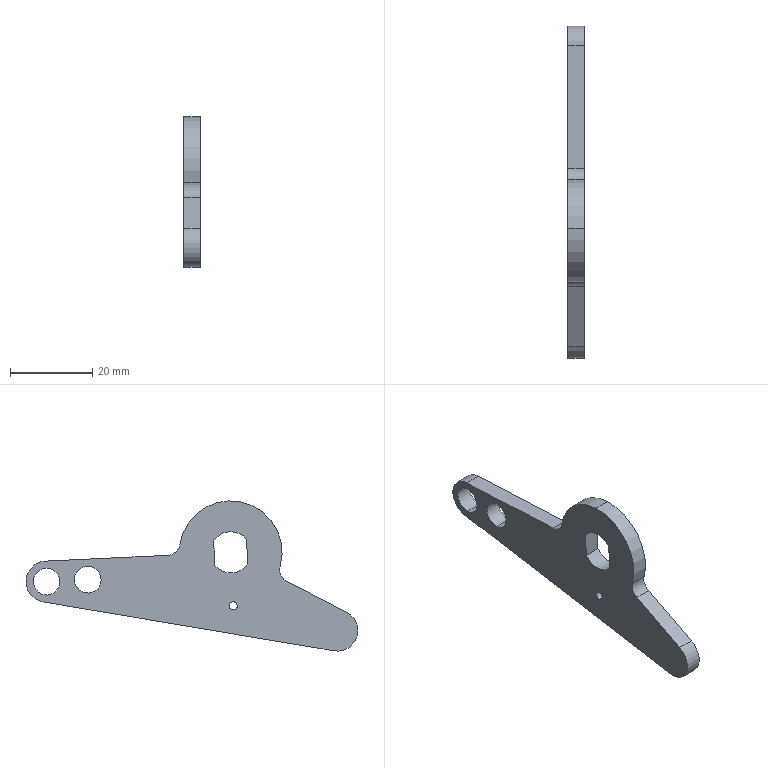Part | SolidWorks | features BaseBody 1 | 1 solid | 22 faces | box 4 x 80.642 x 36.5 mm | volume 5154 mm3 | cylinder 15 | plane 7 | commonest cylinder face diameters 10 x5 6.5 x4 2 x2 6 x2 25 x2
STEP:
#1=CARTESIAN_POINT('',(7.537,-56.512,-203.064));
#2=VERTEX_POINT('',#1);
#3=CARTESIAN_POINT('',(7.537,-69.112,-219.022));
#4=VERTEX_POINT('',#3);
#5=CARTESIAN_POINT('',(7.537,-57.104,-215.55));
#6=DIRECTION('',(1.,0.,0.));
#7=DIRECTION('',(0.,-0.04737,-0.9989));
#8=AXIS2_PLACEMENT_3D('',#5,#6,#7);
#9=CIRCLE('',#8,12.5);
#10=EDGE_CURVE('',#2,#4,#9,.T.);
#11=ORIENTED_EDGE('',*,*,#10,.F.);
#12=CARTESIAN_POINT('',(3.537,-56.512,-203.064));
#13=VERTEX_POINT('',#12);
#14=CARTESIAN_POINT('',(7.537,-56.512,-203.064));
#15=DIRECTION('',(-1.,0.,0.));
#16=VECTOR('',#15,1000.);
#17=LINE('',#14,#16);
#18=EDGE_CURVE('',#2,#13,#17,.T.);
#19=ORIENTED_EDGE('',*,*,#18,.T.);
#20=CARTESIAN_POINT('',(3.537,-69.112,-219.022));
#21=VERTEX_POINT('',#20);
#22=CARTESIAN_POINT('',(3.537,-57.104,-215.55));
#23=DIRECTION('',(1.,0.,0.));
#24=DIRECTION('',(0.,-0.04737,-0.9989));
#25=AXIS2_PLACEMENT_3D('',#22,#23,#24);
#26=CIRCLE('',#25,12.5);
#27=EDGE_CURVE('',#13,#21,#26,.T.);
#28=ORIENTED_EDGE('',*,*,#27,.T.);
#29=CARTESIAN_POINT('',(7.537,-69.112,-219.022));
#30=DIRECTION('',(-1.,0.,0.));
#31=VECTOR('',#30,1000.);
#32=LINE('',#29,#31);
#33=EDGE_CURVE('',#4,#21,#32,.T.);
#34=ORIENTED_EDGE('',*,*,#33,.F.);
#35=EDGE_LOOP('',(#11,#19,#28,#34));
#36=FACE_OUTER_BOUND('',#35,.T.);
#37=CARTESIAN_POINT('',(7.537,-57.104,-215.55));
#38=DIRECTION('',(-1.,0.,0.));
#39=DIRECTION('',(0.,0.04737,0.9989));
#40=AXIS2_PLACEMENT_3D('',#37,#38,#39);
#41=CYLINDRICAL_SURFACE('',#40,12.5);
#42=ADVANCED_FACE('',(#36),#41,.T.);
#43=CARTESIAN_POINT('',(7.537,-52.966,-212.743));
#44=VERTEX_POINT('',#43);
#45=CARTESIAN_POINT('',(7.537,-56.867,-210.556));
#46=VERTEX_POINT('',#45);
#47=CARTESIAN_POINT('',(7.537,-57.104,-215.55));
#48=DIRECTION('',(1.,0.,0.));
#49=DIRECTION('',(0.,-0.04737,-0.9989));
#50=AXIS2_PLACEMENT_3D('',#47,#48,#49);
#51=CIRCLE('',#50,5.);
#52=EDGE_CURVE('',#44,#46,#51,.T.);
#53=ORIENTED_EDGE('',*,*,#52,.T.);
#54=CARTESIAN_POINT('',(3.537,-56.867,-210.556));
#55=VERTEX_POINT('',#54);
#56=CARTESIAN_POINT('',(7.537,-56.867,-210.556));
#57=DIRECTION('',(-1.,0.,0.));
#58=VECTOR('',#57,1000.);
#59=LINE('',#56,#58);
#60=EDGE_CURVE('',#46,#55,#59,.T.);
#61=ORIENTED_EDGE('',*,*,#60,.T.);
#62=CARTESIAN_POINT('',(3.537,-52.966,-212.743));
#63=VERTEX_POINT('',#62);
#64=CARTESIAN_POINT('',(3.537,-57.104,-215.55));
#65=DIRECTION('',(1.,0.,0.));
#66=DIRECTION('',(0.,-0.04737,-0.9989));
#67=AXIS2_PLACEMENT_3D('',#64,#65,#66);
#68=CIRCLE('',#67,5.);
#69=EDGE_CURVE('',#63,#55,#68,.T.);
#70=ORIENTED_EDGE('',*,*,#69,.F.);
#71=CARTESIAN_POINT('',(7.537,-52.966,-212.743));
#72=DIRECTION('',(-1.,0.,0.));
#73=VECTOR('',#72,1000.);
#74=LINE('',#71,#73);
#75=EDGE_CURVE('',#44,#63,#74,.T.);
#76=ORIENTED_EDGE('',*,*,#75,.F.);
#77=EDGE_LOOP('',(#53,#61,#70,#76));
#78=FACE_OUTER_BOUND('',#77,.T.);
#79=CARTESIAN_POINT('',(7.537,-57.104,-215.55));
#80=DIRECTION('',(-1.,0.,0.));
#81=DIRECTION('',(0.,0.04737,0.9989));
#82=AXIS2_PLACEMENT_3D('',#79,#80,#81);
#83=CYLINDRICAL_SURFACE('',#82,5.);
#84=ADVANCED_FACE('',(#78),#83,.F.);
#85=CARTESIAN_POINT('',(7.537,-22.226,-218.956));
#86=VERTEX_POINT('',#85);
#87=CARTESIAN_POINT('',(7.537,-22.534,-225.449));
#88=VERTEX_POINT('',#87);
#89=CARTESIAN_POINT('',(7.537,-22.38,-222.202));
#90=DIRECTION('',(1.,0.,0.));
#91=DIRECTION('',(0.,-0.04737,-0.9989));
#92=AXIS2_PLACEMENT_3D('',#89,#90,#91);
#93=CIRCLE('',#92,3.25);
#94=EDGE_CURVE('',#86,#88,#93,.T.);
#95=ORIENTED_EDGE('',*,*,#94,.T.);
#96=CARTESIAN_POINT('',(3.537,-22.534,-225.449));
#97=VERTEX_POINT('',#96);
#98=CARTESIAN_POINT('',(7.537,-22.534,-225.449));
#99=DIRECTION('',(-1.,0.,0.));
#100=VECTOR('',#99,1000.);
#101=LINE('',#98,#100);
#102=EDGE_CURVE('',#88,#97,#101,.T.);
#103=ORIENTED_EDGE('',*,*,#102,.T.);
#104=CARTESIAN_POINT('',(3.537,-22.226,-218.956));
#105=VERTEX_POINT('',#104);
#106=CARTESIAN_POINT('',(3.537,-22.38,-222.202));
#107=DIRECTION('',(1.,0.,0.));
#108=DIRECTION('',(0.,-0.04737,-0.9989));
#109=AXIS2_PLACEMENT_3D('',#106,#107,#108);
#110=CIRCLE('',#109,3.25);
#111=EDGE_CURVE('',#105,#97,#110,.T.);
#112=ORIENTED_EDGE('',*,*,#111,.F.);
#113=CARTESIAN_POINT('',(7.537,-22.226,-218.956));
#114=DIRECTION('',(-1.,0.,0.));
#115=VECTOR('',#114,1000.);
#116=LINE('',#113,#115);
#117=EDGE_CURVE('',#86,#105,#116,.T.);
#118=ORIENTED_EDGE('',*,*,#117,.F.);
#119=EDGE_LOOP('',(#95,#103,#112,#118));
#120=FACE_OUTER_BOUND('',#119,.T.);
#121=CARTESIAN_POINT('',(7.537,-22.38,-222.202));
#122=DIRECTION('',(-1.,0.,0.));
#123=DIRECTION('',(0.,0.04737,0.9989));
#124=AXIS2_PLACEMENT_3D('',#121,#122,#123);
#125=CYLINDRICAL_SURFACE('',#124,3.25);
#126=ADVANCED_FACE('',(#120),#125,.F.);
#127=CARTESIAN_POINT('',(7.537,-12.237,-219.43));
#128=VERTEX_POINT('',#127);
#129=CARTESIAN_POINT('',(7.537,-12.545,-225.922));
#130=VERTEX_POINT('',#129);
#131=CARTESIAN_POINT('',(7.537,-12.391,-222.676));
#132=DIRECTION('',(1.,0.,0.));
#133=DIRECTION('',(0.,-0.04737,-0.9989));
#134=AXIS2_PLACEMENT_3D('',#131,#132,#133);
#135=CIRCLE('',#134,3.25);
#136=EDGE_CURVE('',#128,#130,#135,.T.);
#137=ORIENTED_EDGE('',*,*,#136,.T.);
#138=CARTESIAN_POINT('',(3.537,-12.545,-225.922));
#139=VERTEX_POINT('',#138);
#140=CARTESIAN_POINT('',(7.537,-12.545,-225.922));
#141=DIRECTION('',(-1.,0.,0.));
#142=VECTOR('',#141,1000.);
#143=LINE('',#140,#142);
#144=EDGE_CURVE('',#130,#139,#143,.T.);
#145=ORIENTED_EDGE('',*,*,#144,.T.);
#146=CARTESIAN_POINT('',(3.537,-12.237,-219.43));
#147=VERTEX_POINT('',#146);
#148=CARTESIAN_POINT('',(3.537,-12.391,-222.676));
#149=DIRECTION('',(1.,0.,0.));
#150=DIRECTION('',(0.,-0.04737,-0.9989));
#151=AXIS2_PLACEMENT_3D('',#148,#149,#150);
#152=CIRCLE('',#151,3.25);
#153=EDGE_CURVE('',#147,#139,#152,.T.);
#154=ORIENTED_EDGE('',*,*,#153,.F.);
#155=CARTESIAN_POINT('',(7.537,-12.237,-219.43));
#156=DIRECTION('',(-1.,0.,0.));
#157=VECTOR('',#156,1000.);
#158=LINE('',#155,#157);
#159=EDGE_CURVE('',#128,#147,#158,.T.);
#160=ORIENTED_EDGE('',*,*,#159,.F.);
#161=EDGE_LOOP('',(#137,#145,#154,#160));
#162=FACE_OUTER_BOUND('',#161,.T.);
#163=CARTESIAN_POINT('',(7.537,-12.391,-222.676));
#164=DIRECTION('',(-1.,0.,0.));
#165=DIRECTION('',(0.,0.04737,0.9989));
#166=AXIS2_PLACEMENT_3D('',#163,#164,#165);
#167=CYLINDRICAL_SURFACE('',#166,3.25);
#168=ADVANCED_FACE('',(#162),#167,.F.);
#169=CARTESIAN_POINT('',(7.537,-57.672,-227.537));
#170=VERTEX_POINT('',#169);
#171=CARTESIAN_POINT('',(7.537,-57.767,-229.534));
#172=VERTEX_POINT('',#171);
#173=CARTESIAN_POINT('',(7.537,-57.72,-228.535));
#174=DIRECTION('',(1.,0.,0.));
#175=DIRECTION('',(0.,-0.04737,-0.9989));
#176=AXIS2_PLACEMENT_3D('',#173,#174,#175);
#177=CIRCLE('',#176,1.);
#178=EDGE_CURVE('',#170,#172,#177,.T.);
#179=ORIENTED_EDGE('',*,*,#178,.T.);
#180=CARTESIAN_POINT('',(3.537,-57.767,-229.534));
#181=VERTEX_POINT('',#180);
#182=CARTESIAN_POINT('',(7.537,-57.767,-229.534));
#183=DIRECTION('',(-1.,0.,0.));
#184=VECTOR('',#183,1000.);
#185=LINE('',#182,#184);
#186=EDGE_CURVE('',#172,#181,#185,.T.);
#187=ORIENTED_EDGE('',*,*,#186,.T.);
#188=CARTESIAN_POINT('',(3.537,-57.672,-227.537));
#189=VERTEX_POINT('',#188);
#190=CARTESIAN_POINT('',(3.537,-57.72,-228.535));
#191=DIRECTION('',(1.,0.,0.));
#192=DIRECTION('',(0.,-0.04737,-0.9989));
#193=AXIS2_PLACEMENT_3D('',#190,#191,#192);
#194=CIRCLE('',#193,1.);
#195=EDGE_CURVE('',#189,#181,#194,.T.);
#196=ORIENTED_EDGE('',*,*,#195,.F.);
#197=CARTESIAN_POINT('',(7.537,-57.672,-227.537));
#198=DIRECTION('',(-1.,0.,0.));
#199=VECTOR('',#198,1000.);
#200=LINE('',#197,#199);
#201=EDGE_CURVE('',#170,#189,#200,.T.);
#202=ORIENTED_EDGE('',*,*,#201,.F.);
#203=EDGE_LOOP('',(#179,#187,#196,#202));
#204=FACE_OUTER_BOUND('',#203,.T.);
#205=CARTESIAN_POINT('',(7.537,-57.72,-228.535));
#206=DIRECTION('',(-1.,0.,0.));
#207=DIRECTION('',(0.,0.04737,0.9989));
#208=AXIS2_PLACEMENT_3D('',#205,#206,#207);
#209=CYLINDRICAL_SURFACE('',#208,1.);
#210=ADVANCED_FACE('',(#204),#209,.F.);
#211=ORIENTED_EDGE('',*,*,#186,.F.);
#212=CARTESIAN_POINT('',(7.537,-57.72,-228.535));
#213=DIRECTION('',(1.,0.,0.));
#214=DIRECTION('',(0.,-0.04737,-0.9989));
#215=AXIS2_PLACEMENT_3D('',#212,#213,#214);
#216=CIRCLE('',#215,1.);
#217=EDGE_CURVE('',#172,#170,#216,.T.);
#218=ORIENTED_EDGE('',*,*,#217,.T.);
#219=ORIENTED_EDGE('',*,*,#201,.T.);
#220=CARTESIAN_POINT('',(3.537,-57.72,-228.535));
#221=DIRECTION('',(1.,0.,0.));
#222=DIRECTION('',(0.,-0.04737,-0.9989));
#223=AXIS2_PLACEMENT_3D('',#220,#221,#222);
#224=CIRCLE('',#223,1.);
#225=EDGE_CURVE('',#181,#189,#224,.T.);
#226=ORIENTED_EDGE('',*,*,#225,.F.);
#227=EDGE_LOOP('',(#211,#218,#219,#226));
#228=FACE_OUTER_BOUND('',#227,.T.);
#229=CARTESIAN_POINT('',(7.537,-57.72,-228.535));
#230=DIRECTION('',(-1.,0.,0.));
#231=DIRECTION('',(0.,0.04737,0.9989));
#232=AXIS2_PLACEMENT_3D('',#229,#230,#231);
#233=CYLINDRICAL_SURFACE('',#232,1.);
#234=ADVANCED_FACE('',(#228),#233,.F.);
#235=ORIENTED_EDGE('',*,*,#144,.F.);
#236=CARTESIAN_POINT('',(7.537,-12.391,-222.676));
#237=DIRECTION('',(1.,0.,0.));
#238=DIRECTION('',(0.,-0.04737,-0.9989));
#239=AXIS2_PLACEMENT_3D('',#236,#237,#238);
#240=CIRCLE('',#239,3.25);
#241=EDGE_CURVE('',#130,#128,#240,.T.);
#242=ORIENTED_EDGE('',*,*,#241,.T.);
#243=ORIENTED_EDGE('',*,*,#159,.T.);
#244=CARTESIAN_POINT('',(3.537,-12.391,-222.676));
#245=DIRECTION('',(1.,0.,0.));
#246=DIRECTION('',(0.,-0.04737,-0.9989));
#247=AXIS2_PLACEMENT_3D('',#244,#245,#246);
#248=CIRCLE('',#247,3.25);
#249=EDGE_CURVE('',#139,#147,#248,.T.);
#250=ORIENTED_EDGE('',*,*,#249,.F.);
#251=EDGE_LOOP('',(#235,#242,#243,#250));
#252=FACE_OUTER_BOUND('',#251,.T.);
#253=CARTESIAN_POINT('',(7.537,-12.391,-222.676));
#254=DIRECTION('',(-1.,0.,0.));
#255=DIRECTION('',(0.,0.04737,0.9989));
#256=AXIS2_PLACEMENT_3D('',#253,#254,#255);
#257=CYLINDRICAL_SURFACE('',#256,3.25);
#258=ADVANCED_FACE('',(#252),#257,.F.);
#259=ORIENTED_EDGE('',*,*,#102,.F.);
#260=CARTESIAN_POINT('',(7.537,-22.38,-222.202));
#261=DIRECTION('',(1.,0.,0.));
#262=DIRECTION('',(0.,-0.04737,-0.9989));
#263=AXIS2_PLACEMENT_3D('',#260,#261,#262);
#264=CIRCLE('',#263,3.25);
#265=EDGE_CURVE('',#88,#86,#264,.T.);
#266=ORIENTED_EDGE('',*,*,#265,.T.);
#267=ORIENTED_EDGE('',*,*,#117,.T.);
#268=CARTESIAN_POINT('',(3.537,-22.38,-222.202));
#269=DIRECTION('',(1.,0.,0.));
#270=DIRECTION('',(0.,-0.04737,-0.9989));
#271=AXIS2_PLACEMENT_3D('',#268,#269,#270);
#272=CIRCLE('',#271,3.25);
#273=EDGE_CURVE('',#97,#105,#272,.T.);
#274=ORIENTED_EDGE('',*,*,#273,.F.);
#275=EDGE_LOOP('',(#259,#266,#267,#274));
#276=FACE_OUTER_BOUND('',#275,.T.);
#277=CARTESIAN_POINT('',(7.537,-22.38,-222.202));
#278=DIRECTION('',(-1.,0.,0.));
#279=DIRECTION('',(0.,0.04737,0.9989));
#280=AXIS2_PLACEMENT_3D('',#277,#278,#279);
#281=CYLINDRICAL_SURFACE('',#280,3.25);
#282=ADVANCED_FACE('',(#276),#281,.F.);
#283=CARTESIAN_POINT('',(3.537,-53.25,-218.736));
#284=VERTEX_POINT('',#283);
#285=CARTESIAN_POINT('',(3.537,-52.966,-212.743));
#286=DIRECTION('',(0.,0.04737,0.9989));
#287=VECTOR('',#286,1000.);
#288=LINE('',#285,#287);
#289=EDGE_CURVE('',#284,#63,#288,.T.);
#290=ORIENTED_EDGE('',*,*,#289,.F.);
#291=CARTESIAN_POINT('',(7.537,-53.25,-218.736));
#292=VERTEX_POINT('',#291);
#293=CARTESIAN_POINT('',(7.537,-53.25,-218.736));
#294=DIRECTION('',(-1.,0.,0.));
#295=VECTOR('',#294,1000.);
#296=LINE('',#293,#295);
#297=EDGE_CURVE('',#292,#284,#296,.T.);
#298=ORIENTED_EDGE('',*,*,#297,.F.);
#299=CARTESIAN_POINT('',(7.537,-52.966,-212.743));
#300=DIRECTION('',(0.,0.04737,0.9989));
#301=VECTOR('',#300,1000.);
#302=LINE('',#299,#301);
#303=EDGE_CURVE('',#292,#44,#302,.T.);
#304=ORIENTED_EDGE('',*,*,#303,.T.);
#305=ORIENTED_EDGE('',*,*,#75,.T.);
#306=EDGE_LOOP('',(#290,#298,#304,#305));
#307=FACE_OUTER_BOUND('',#306,.T.);
#308=CARTESIAN_POINT('',(7.537,-52.966,-212.743));
#309=DIRECTION('',(0.,-0.9989,0.04737));
#310=DIRECTION('',(-1.,0.,0.));
#311=AXIS2_PLACEMENT_3D('',#308,#309,#310);
#312=PLANE('',#311);
#313=ADVANCED_FACE('',(#307),#312,.T.);
#314=CARTESIAN_POINT('',(3.537,-61.241,-218.357));
#315=VERTEX_POINT('',#314);
#316=CARTESIAN_POINT('',(3.537,-57.104,-215.55));
#317=DIRECTION('',(1.,0.,0.));
#318=DIRECTION('',(0.,-0.04737,-0.9989));
#319=AXIS2_PLACEMENT_3D('',#316,#317,#318);
#320=CIRCLE('',#319,5.);
#321=EDGE_CURVE('',#315,#284,#320,.T.);
#322=ORIENTED_EDGE('',*,*,#321,.F.);
#323=CARTESIAN_POINT('',(7.537,-61.241,-218.357));
#324=VERTEX_POINT('',#323);
#325=CARTESIAN_POINT('',(7.537,-61.241,-218.357));
#326=DIRECTION('',(-1.,0.,0.));
#327=VECTOR('',#326,1000.);
#328=LINE('',#325,#327);
#329=EDGE_CURVE('',#324,#315,#328,.T.);
#330=ORIENTED_EDGE('',*,*,#329,.F.);
#331=CARTESIAN_POINT('',(7.537,-57.104,-215.55));
#332=DIRECTION('',(1.,0.,0.));
#333=DIRECTION('',(0.,-0.04737,-0.9989));
#334=AXIS2_PLACEMENT_3D('',#331,#332,#333);
#335=CIRCLE('',#334,5.);
#336=EDGE_CURVE('',#324,#292,#335,.T.);
#337=ORIENTED_EDGE('',*,*,#336,.T.);
#338=ORIENTED_EDGE('',*,*,#297,.T.);
#339=EDGE_LOOP('',(#322,#330,#337,#338));
#340=FACE_OUTER_BOUND('',#339,.T.);
#341=CARTESIAN_POINT('',(7.537,-57.104,-215.55));
#342=DIRECTION('',(-1.,0.,0.));
#343=DIRECTION('',(0.,0.04737,0.9989));
#344=AXIS2_PLACEMENT_3D('',#341,#342,#343);
#345=CYLINDRICAL_SURFACE('',#344,5.);
#346=ADVANCED_FACE('',(#340),#345,.F.);
#347=CARTESIAN_POINT('',(3.537,-60.957,-212.364));
#348=VERTEX_POINT('',#347);
#349=CARTESIAN_POINT('',(3.537,-60.957,-212.364));
#350=DIRECTION('',(0.,-0.04737,-0.9989));
#351=VECTOR('',#350,1000.);
#352=LINE('',#349,#351);
#353=EDGE_CURVE('',#348,#315,#352,.T.);
#354=ORIENTED_EDGE('',*,*,#353,.F.);
#355=CARTESIAN_POINT('',(7.537,-60.957,-212.364));
#356=VERTEX_POINT('',#355);
#357=CARTESIAN_POINT('',(7.537,-60.957,-212.364));
#358=DIRECTION('',(-1.,0.,0.));
#359=VECTOR('',#358,1000.);
#360=LINE('',#357,#359);
#361=EDGE_CURVE('',#356,#348,#360,.T.);
#362=ORIENTED_EDGE('',*,*,#361,.F.);
#363=CARTESIAN_POINT('',(7.537,-60.957,-212.364));
#364=DIRECTION('',(0.,-0.04737,-0.9989));
#365=VECTOR('',#364,1000.);
#366=LINE('',#363,#365);
#367=EDGE_CURVE('',#356,#324,#366,.T.);
#368=ORIENTED_EDGE('',*,*,#367,.T.);
#369=ORIENTED_EDGE('',*,*,#329,.T.);
#370=EDGE_LOOP('',(#354,#362,#368,#369));
#371=FACE_OUTER_BOUND('',#370,.T.);
#372=CARTESIAN_POINT('',(7.537,-60.957,-212.364));
#373=DIRECTION('',(0.,0.9989,-0.04737));
#374=DIRECTION('',(-1.,0.,0.));
#375=AXIS2_PLACEMENT_3D('',#372,#373,#374);
#376=PLANE('',#375);
#377=ADVANCED_FACE('',(#371),#376,.T.);
#378=ORIENTED_EDGE('',*,*,#60,.F.);
#379=CARTESIAN_POINT('',(7.537,-57.104,-215.55));
#380=DIRECTION('',(1.,0.,0.));
#381=DIRECTION('',(0.,-0.04737,-0.9989));
#382=AXIS2_PLACEMENT_3D('',#379,#380,#381);
#383=CIRCLE('',#382,5.);
#384=EDGE_CURVE('',#46,#356,#383,.T.);
#385=ORIENTED_EDGE('',*,*,#384,.T.);
#386=ORIENTED_EDGE('',*,*,#361,.T.);
#387=CARTESIAN_POINT('',(3.537,-57.104,-215.55));
#388=DIRECTION('',(1.,0.,0.));
#389=DIRECTION('',(0.,-0.04737,-0.9989));
#390=AXIS2_PLACEMENT_3D('',#387,#388,#389);
#391=CIRCLE('',#390,5.);
#392=EDGE_CURVE('',#55,#348,#391,.T.);
#393=ORIENTED_EDGE('',*,*,#392,.F.);
#394=EDGE_LOOP('',(#378,#385,#386,#393));
#395=FACE_OUTER_BOUND('',#394,.T.);
#396=CARTESIAN_POINT('',(7.537,-57.104,-215.55));
#397=DIRECTION('',(-1.,0.,0.));
#398=DIRECTION('',(0.,0.04737,0.9989));
#399=AXIS2_PLACEMENT_3D('',#396,#397,#398);
#400=CYLINDRICAL_SURFACE('',#399,5.);
#401=ADVANCED_FACE('',(#395),#400,.F.);
#402=CARTESIAN_POINT('',(3.537,-82.204,-239.481));
#403=VERTEX_POINT('',#402);
#404=CARTESIAN_POINT('',(3.537,-11.562,-227.607));
#405=VERTEX_POINT('',#404);
#406=CARTESIAN_POINT('',(3.537,-11.562,-227.607));
#407=DIRECTION('',(0.,0.9862,0.1658));
#408=VECTOR('',#407,1000.);
#409=LINE('',#406,#408);
#410=EDGE_CURVE('',#403,#405,#409,.T.);
#411=ORIENTED_EDGE('',*,*,#410,.T.);
#412=CARTESIAN_POINT('',(7.537,-11.562,-227.607));
#413=VERTEX_POINT('',#412);
#414=CARTESIAN_POINT('',(7.537,-11.562,-227.607));
#415=DIRECTION('',(-1.,0.,0.));
#416=VECTOR('',#415,1000.);
#417=LINE('',#414,#416);
#418=EDGE_CURVE('',#413,#405,#417,.T.);
#419=ORIENTED_EDGE('',*,*,#418,.F.);
#420=CARTESIAN_POINT('',(7.537,-82.204,-239.481));
#421=VERTEX_POINT('',#420);
#422=CARTESIAN_POINT('',(7.537,-11.562,-227.607));
#423=DIRECTION('',(0.,0.9862,0.1658));
#424=VECTOR('',#423,1000.);
#425=LINE('',#422,#424);
#426=EDGE_CURVE('',#421,#413,#425,.T.);
#427=ORIENTED_EDGE('',*,*,#426,.F.);
#428=CARTESIAN_POINT('',(7.537,-82.204,-239.481));
#429=DIRECTION('',(-1.,0.,0.));
#430=VECTOR('',#429,1000.);
#431=LINE('',#428,#430);
#432=EDGE_CURVE('',#421,#403,#431,.T.);
#433=ORIENTED_EDGE('',*,*,#432,.T.);
#434=EDGE_LOOP('',(#411,#419,#427,#433));
#435=FACE_OUTER_BOUND('',#434,.T.);
#436=CARTESIAN_POINT('',(7.537,-11.562,-227.607));
#437=DIRECTION('',(0.,-0.1658,0.9862));
#438=DIRECTION('',(-1.,0.,0.));
#439=AXIS2_PLACEMENT_3D('',#436,#437,#438);
#440=PLANE('',#439);
#441=ADVANCED_FACE('',(#435),#440,.F.);
#442=CARTESIAN_POINT('',(3.537,-85.325,-230.107));
#443=VERTEX_POINT('',#442);
#444=CARTESIAN_POINT('',(3.537,-83.033,-234.55));
#445=DIRECTION('',(1.,0.,0.));
#446=DIRECTION('',(0.,-0.04737,-0.9989));
#447=AXIS2_PLACEMENT_3D('',#444,#445,#446);
#448=CIRCLE('',#447,5.);
#449=EDGE_CURVE('',#443,#403,#448,.T.);
#450=ORIENTED_EDGE('',*,*,#449,.T.);
#451=ORIENTED_EDGE('',*,*,#432,.F.);
#452=CARTESIAN_POINT('',(7.537,-85.325,-230.107));
#453=VERTEX_POINT('',#452);
#454=CARTESIAN_POINT('',(7.537,-83.033,-234.55));
#455=DIRECTION('',(1.,0.,0.));
#456=DIRECTION('',(0.,-0.04737,-0.9989));
#457=AXIS2_PLACEMENT_3D('',#454,#455,#456);
#458=CIRCLE('',#457,5.);
#459=EDGE_CURVE('',#453,#421,#458,.T.);
#460=ORIENTED_EDGE('',*,*,#459,.F.);
#461=CARTESIAN_POINT('',(7.537,-85.325,-230.107));
#462=DIRECTION('',(-1.,0.,0.));
#463=VECTOR('',#462,1000.);
#464=LINE('',#461,#463);
#465=EDGE_CURVE('',#453,#443,#464,.T.);
#466=ORIENTED_EDGE('',*,*,#465,.T.);
#467=EDGE_LOOP('',(#450,#451,#460,#466));
#468=FACE_OUTER_BOUND('',#467,.T.);
#469=CARTESIAN_POINT('',(7.537,-83.033,-234.55));
#470=DIRECTION('',(-1.,0.,0.));
#471=DIRECTION('',(0.,0.04737,0.9989));
#472=AXIS2_PLACEMENT_3D('',#469,#470,#471);
#473=CYLINDRICAL_SURFACE('',#472,5.);
#474=ADVANCED_FACE('',(#468),#473,.T.);
#475=CARTESIAN_POINT('',(3.537,-70.619,-222.521));
#476=VERTEX_POINT('',#475);
#477=CARTESIAN_POINT('',(3.537,-70.619,-222.521));
#478=DIRECTION('',(0.,-0.8887,-0.4584));
#479=VECTOR('',#478,1000.);
#480=LINE('',#477,#479);
#481=EDGE_CURVE('',#476,#443,#480,.T.);
#482=ORIENTED_EDGE('',*,*,#481,.T.);
#483=ORIENTED_EDGE('',*,*,#465,.F.);
#484=CARTESIAN_POINT('',(7.537,-70.619,-222.521));
#485=VERTEX_POINT('',#484);
#486=CARTESIAN_POINT('',(7.537,-70.619,-222.521));
#487=DIRECTION('',(0.,-0.8887,-0.4584));
#488=VECTOR('',#487,1000.);
#489=LINE('',#486,#488);
#490=EDGE_CURVE('',#485,#453,#489,.T.);
#491=ORIENTED_EDGE('',*,*,#490,.F.);
#492=CARTESIAN_POINT('',(7.537,-70.619,-222.521));
#493=DIRECTION('',(-1.,0.,0.));
#494=VECTOR('',#493,1000.);
#495=LINE('',#492,#494);
#496=EDGE_CURVE('',#485,#476,#495,.T.);
#497=ORIENTED_EDGE('',*,*,#496,.T.);
#498=EDGE_LOOP('',(#482,#483,#491,#497));
#499=FACE_OUTER_BOUND('',#498,.T.);
#500=CARTESIAN_POINT('',(7.537,-70.619,-222.521));
#501=DIRECTION('',(0.,0.4584,-0.8887));
#502=DIRECTION('',(-1.,0.,0.));
#503=AXIS2_PLACEMENT_3D('',#500,#501,#502);
#504=PLANE('',#503);
#505=ADVANCED_FACE('',(#499),#504,.F.);
#506=CARTESIAN_POINT('',(3.537,-71.994,-219.855));
#507=DIRECTION('',(-1.,0.,0.));
#508=DIRECTION('',(0.,0.04737,0.9989));
#509=AXIS2_PLACEMENT_3D('',#506,#507,#508);
#510=CIRCLE('',#509,3.);
#511=EDGE_CURVE('',#21,#476,#510,.T.);
#512=ORIENTED_EDGE('',*,*,#511,.T.);
#513=ORIENTED_EDGE('',*,*,#496,.F.);
#514=CARTESIAN_POINT('',(7.537,-71.994,-219.855));
#515=DIRECTION('',(-1.,0.,0.));
#516=DIRECTION('',(0.,0.04737,0.9989));
#517=AXIS2_PLACEMENT_3D('',#514,#515,#516);
#518=CIRCLE('',#517,3.);
#519=EDGE_CURVE('',#4,#485,#518,.T.);
#520=ORIENTED_EDGE('',*,*,#519,.F.);
#521=ORIENTED_EDGE('',*,*,#33,.T.);
#522=EDGE_LOOP('',(#512,#513,#520,#521));
#523=FACE_OUTER_BOUND('',#522,.T.);
#524=CARTESIAN_POINT('',(7.537,-71.994,-219.855));
#525=DIRECTION('',(-1.,0.,0.));
#526=DIRECTION('',(0.,0.04737,0.9989));
#527=AXIS2_PLACEMENT_3D('',#524,#525,#526);
#528=CYLINDRICAL_SURFACE('',#527,3.);
#529=ADVANCED_FACE('',(#523),#528,.F.);
#530=ORIENTED_EDGE('',*,*,#18,.F.);
#531=CARTESIAN_POINT('',(7.537,-44.739,-213.714));
#532=VERTEX_POINT('',#531);
#533=CARTESIAN_POINT('',(7.537,-57.104,-215.55));
#534=DIRECTION('',(1.,0.,0.));
#535=DIRECTION('',(0.,-0.04737,-0.9989));
#536=AXIS2_PLACEMENT_3D('',#533,#534,#535);
#537=CIRCLE('',#536,12.5);
#538=EDGE_CURVE('',#532,#2,#537,.T.);
#539=ORIENTED_EDGE('',*,*,#538,.F.);
#540=CARTESIAN_POINT('',(3.537,-44.739,-213.714));
#541=VERTEX_POINT('',#540);
#542=CARTESIAN_POINT('',(7.537,-44.739,-213.714));
#543=DIRECTION('',(-1.,0.,0.));
#544=VECTOR('',#543,1000.);
#545=LINE('',#542,#544);
#546=EDGE_CURVE('',#532,#541,#545,.T.);
#547=ORIENTED_EDGE('',*,*,#546,.T.);
#548=CARTESIAN_POINT('',(3.537,-57.104,-215.55));
#549=DIRECTION('',(1.,0.,0.));
#550=DIRECTION('',(0.,-0.04737,-0.9989));
#551=AXIS2_PLACEMENT_3D('',#548,#549,#550);
#552=CIRCLE('',#551,12.5);
#553=EDGE_CURVE('',#541,#13,#552,.T.);
#554=ORIENTED_EDGE('',*,*,#553,.T.);
#555=EDGE_LOOP('',(#530,#539,#547,#554));
#556=FACE_OUTER_BOUND('',#555,.T.);
#557=CARTESIAN_POINT('',(7.537,-57.104,-215.55));
#558=DIRECTION('',(-1.,0.,0.));
#559=DIRECTION('',(0.,0.04737,0.9989));
#560=AXIS2_PLACEMENT_3D('',#557,#558,#559);
#561=CYLINDRICAL_SURFACE('',#560,12.5);
#562=ADVANCED_FACE('',(#556),#561,.T.);
#563=CARTESIAN_POINT('',(3.537,-41.914,-216.27));
#564=VERTEX_POINT('',#563);
#565=CARTESIAN_POINT('',(3.537,-41.772,-213.274));
#566=DIRECTION('',(-1.,0.,0.));
#567=DIRECTION('',(0.,0.04737,0.9989));
#568=AXIS2_PLACEMENT_3D('',#565,#566,#567);
#569=CIRCLE('',#568,3.);
#570=EDGE_CURVE('',#564,#541,#569,.T.);
#571=ORIENTED_EDGE('',*,*,#570,.T.);
#572=ORIENTED_EDGE('',*,*,#546,.F.);
#573=CARTESIAN_POINT('',(7.537,-41.914,-216.27));
#574=VERTEX_POINT('',#573);
#575=CARTESIAN_POINT('',(7.537,-41.772,-213.274));
#576=DIRECTION('',(-1.,0.,0.));
#577=DIRECTION('',(0.,0.04737,0.9989));
#578=AXIS2_PLACEMENT_3D('',#575,#576,#577);
#579=CIRCLE('',#578,3.);
#580=EDGE_CURVE('',#574,#532,#579,.T.);
#581=ORIENTED_EDGE('',*,*,#580,.F.);
#582=CARTESIAN_POINT('',(7.537,-41.914,-216.27));
#583=DIRECTION('',(-1.,0.,0.));
#584=VECTOR('',#583,1000.);
#585=LINE('',#582,#584);
#586=EDGE_CURVE('',#574,#564,#585,.T.);
#587=ORIENTED_EDGE('',*,*,#586,.T.);
#588=EDGE_LOOP('',(#571,#572,#581,#587));
#589=FACE_OUTER_BOUND('',#588,.T.);
#590=CARTESIAN_POINT('',(7.537,-41.772,-213.274));
#591=DIRECTION('',(-1.,0.,0.));
#592=DIRECTION('',(0.,0.04737,0.9989));
#593=AXIS2_PLACEMENT_3D('',#590,#591,#592);
#594=CYLINDRICAL_SURFACE('',#593,3.);
#595=ADVANCED_FACE('',(#589),#594,.F.);
#596=CARTESIAN_POINT('',(3.537,-12.154,-217.682));
#597=VERTEX_POINT('',#596);
#598=CARTESIAN_POINT('',(3.537,-12.154,-217.682));
#599=DIRECTION('',(0.,-0.9989,0.04737));
#600=VECTOR('',#599,1000.);
#601=LINE('',#598,#600);
#602=EDGE_CURVE('',#597,#564,#601,.T.);
#603=ORIENTED_EDGE('',*,*,#602,.T.);
#604=ORIENTED_EDGE('',*,*,#586,.F.);
#605=CARTESIAN_POINT('',(7.537,-12.154,-217.682));
#606=VERTEX_POINT('',#605);
#607=CARTESIAN_POINT('',(7.537,-12.154,-217.682));
#608=DIRECTION('',(0.,-0.9989,0.04737));
#609=VECTOR('',#608,1000.);
#610=LINE('',#607,#609);
#611=EDGE_CURVE('',#606,#574,#610,.T.);
#612=ORIENTED_EDGE('',*,*,#611,.F.);
#613=CARTESIAN_POINT('',(7.537,-12.154,-217.682));
#614=DIRECTION('',(-1.,0.,0.));
#615=VECTOR('',#614,1000.);
#616=LINE('',#613,#615);
#617=EDGE_CURVE('',#606,#597,#616,.T.);
#618=ORIENTED_EDGE('',*,*,#617,.T.);
#619=EDGE_LOOP('',(#603,#604,#612,#618));
#620=FACE_OUTER_BOUND('',#619,.T.);
#621=CARTESIAN_POINT('',(7.537,-12.154,-217.682));
#622=DIRECTION('',(0.,-0.04737,-0.9989));
#623=DIRECTION('',(0.,-0.9989,0.04737));
#624=AXIS2_PLACEMENT_3D('',#621,#622,#623);
#625=PLANE('',#624);
#626=ADVANCED_FACE('',(#620),#625,.F.);
#627=CARTESIAN_POINT('',(3.537,-12.391,-222.676));
#628=DIRECTION('',(1.,0.,0.));
#629=DIRECTION('',(0.,-0.04737,-0.9989));
#630=AXIS2_PLACEMENT_3D('',#627,#628,#629);
#631=CIRCLE('',#630,5.);
#632=EDGE_CURVE('',#405,#597,#631,.T.);
#633=ORIENTED_EDGE('',*,*,#632,.T.);
#634=ORIENTED_EDGE('',*,*,#617,.F.);
#635=CARTESIAN_POINT('',(7.537,-12.391,-222.676));
#636=DIRECTION('',(1.,0.,0.));
#637=DIRECTION('',(0.,-0.04737,-0.9989));
#638=AXIS2_PLACEMENT_3D('',#635,#636,#637);
#639=CIRCLE('',#638,5.);
#640=EDGE_CURVE('',#413,#606,#639,.T.);
#641=ORIENTED_EDGE('',*,*,#640,.F.);
#642=ORIENTED_EDGE('',*,*,#418,.T.);
#643=EDGE_LOOP('',(#633,#634,#641,#642));
#644=FACE_OUTER_BOUND('',#643,.T.);
#645=CARTESIAN_POINT('',(7.537,-12.391,-222.676));
#646=DIRECTION('',(-1.,0.,0.));
#647=DIRECTION('',(0.,0.04737,0.9989));
#648=AXIS2_PLACEMENT_3D('',#645,#646,#647);
#649=CYLINDRICAL_SURFACE('',#648,5.);
#650=ADVANCED_FACE('',(#644),#649,.T.);
#651=ORIENTED_EDGE('',*,*,#195,.T.);
#652=ORIENTED_EDGE('',*,*,#225,.T.);
#653=EDGE_LOOP('',(#651,#652));
#654=FACE_BOUND('',#653,.T.);
#655=ORIENTED_EDGE('',*,*,#111,.T.);
#656=ORIENTED_EDGE('',*,*,#273,.T.);
#657=EDGE_LOOP('',(#655,#656));
#658=FACE_BOUND('',#657,.T.);
#659=ORIENTED_EDGE('',*,*,#632,.F.);
#660=ORIENTED_EDGE('',*,*,#410,.F.);
#661=ORIENTED_EDGE('',*,*,#449,.F.);
#662=ORIENTED_EDGE('',*,*,#481,.F.);
#663=ORIENTED_EDGE('',*,*,#511,.F.);
#664=ORIENTED_EDGE('',*,*,#27,.F.);
#665=ORIENTED_EDGE('',*,*,#553,.F.);
#666=ORIENTED_EDGE('',*,*,#570,.F.);
#667=ORIENTED_EDGE('',*,*,#602,.F.);
#668=EDGE_LOOP('',(#659,#660,#661,#662,#663,#664,#665,#666,#667));
#669=FACE_OUTER_BOUND('',#668,.T.);
#670=ORIENTED_EDGE('',*,*,#69,.T.);
#671=ORIENTED_EDGE('',*,*,#392,.T.);
#672=ORIENTED_EDGE('',*,*,#353,.T.);
#673=ORIENTED_EDGE('',*,*,#321,.T.);
#674=ORIENTED_EDGE('',*,*,#289,.T.);
#675=EDGE_LOOP('',(#670,#671,#672,#673,#674));
#676=FACE_BOUND('',#675,.T.);
#677=ORIENTED_EDGE('',*,*,#153,.T.);
#678=ORIENTED_EDGE('',*,*,#249,.T.);
#679=EDGE_LOOP('',(#677,#678));
#680=FACE_BOUND('',#679,.T.);
#681=CARTESIAN_POINT('',(3.537,-12.391,-222.676));
#682=DIRECTION('',(1.,0.,0.));
#683=DIRECTION('',(0.,0.,-1.));
#684=AXIS2_PLACEMENT_3D('',#681,#682,#683);
#685=PLANE('',#684);
#686=ADVANCED_FACE('',(#654,#658,#669,#676,#680),#685,.F.);
#687=ORIENTED_EDGE('',*,*,#178,.F.);
#688=ORIENTED_EDGE('',*,*,#217,.F.);
#689=EDGE_LOOP('',(#687,#688));
#690=FACE_BOUND('',#689,.T.);
#691=ORIENTED_EDGE('',*,*,#94,.F.);
#692=ORIENTED_EDGE('',*,*,#265,.F.);
#693=EDGE_LOOP('',(#691,#692));
#694=FACE_BOUND('',#693,.T.);
#695=ORIENTED_EDGE('',*,*,#640,.T.);
#696=ORIENTED_EDGE('',*,*,#611,.T.);
#697=ORIENTED_EDGE('',*,*,#580,.T.);
#698=ORIENTED_EDGE('',*,*,#538,.T.);
#699=ORIENTED_EDGE('',*,*,#10,.T.);
#700=ORIENTED_EDGE('',*,*,#519,.T.);
#701=ORIENTED_EDGE('',*,*,#490,.T.);
#702=ORIENTED_EDGE('',*,*,#459,.T.);
#703=ORIENTED_EDGE('',*,*,#426,.T.);
#704=EDGE_LOOP('',(#695,#696,#697,#698,#699,#700,#701,#702,#703));
#705=FACE_OUTER_BOUND('',#704,.T.);
#706=ORIENTED_EDGE('',*,*,#367,.F.);
#707=ORIENTED_EDGE('',*,*,#384,.F.);
#708=ORIENTED_EDGE('',*,*,#52,.F.);
#709=ORIENTED_EDGE('',*,*,#303,.F.);
#710=ORIENTED_EDGE('',*,*,#336,.F.);
#711=EDGE_LOOP('',(#706,#707,#708,#709,#710));
#712=FACE_BOUND('',#711,.T.);
#713=ORIENTED_EDGE('',*,*,#136,.F.);
#714=ORIENTED_EDGE('',*,*,#241,.F.);
#715=EDGE_LOOP('',(#713,#714));
#716=FACE_BOUND('',#715,.T.);
#717=CARTESIAN_POINT('',(7.537,-12.391,-222.676));
#718=DIRECTION('',(1.,0.,0.));
#719=DIRECTION('',(0.,0.,-1.));
#720=AXIS2_PLACEMENT_3D('',#717,#718,#719);
#721=PLANE('',#720);
#722=ADVANCED_FACE('',(#690,#694,#705,#712,#716),#721,.T.);
#723=CLOSED_SHELL('',(#42,#84,#126,#168,#210,#234,#258,#282,#313,#346,#377,#401,#441,#474,#505,#529,#562,#595,#626,#650,#686,#722));
#724=MANIFOLD_SOLID_BREP('',#723);
#725=CARTESIAN_POINT('',(0.,0.,0.));
#726=DIRECTION('',(0.,0.,1.));
#727=DIRECTION('',(1.,0.,0.));
#728=AXIS2_PLACEMENT_3D('',#725,#726,#727);
#729=(LENGTH_UNIT()NAMED_UNIT(*)SI_UNIT(.MILLI.,.METRE.));
#730=UNCERTAINTY_MEASURE_WITH_UNIT(LENGTH_MEASURE(0.00001),#729,'','');
#731=(NAMED_UNIT(*)PLANE_ANGLE_UNIT()SI_UNIT($,.RADIAN.));
#732=(NAMED_UNIT(*)SI_UNIT($,.STERADIAN.)SOLID_ANGLE_UNIT());
#733=(GEOMETRIC_REPRESENTATION_CONTEXT(3)GLOBAL_UNCERTAINTY_ASSIGNED_CONTEXT((#730))GLOBAL_UNIT_ASSIGNED_CONTEXT((#729,#731,#732))REPRESENTATION_CONTEXT('',''));
#734=ADVANCED_BREP_SHAPE_REPRESENTATION('',(#724,#728),#733);